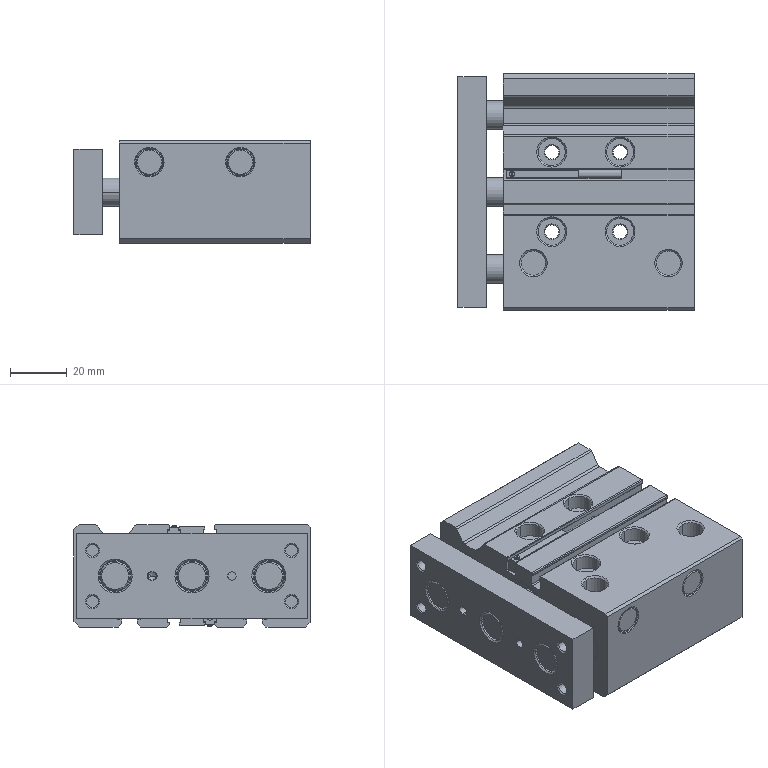Part | SolidWorks | 4 solids | 443 faces | box 83 x 83 x 36 mm | volume 177005 mm3 | cylinder 185 | plane 150 | cone 106 | torus 2 | commonest cylinder face diameters 3 x25 0.8 x20 0.4 x16 4.134 x16 0.6 x14 10 x12